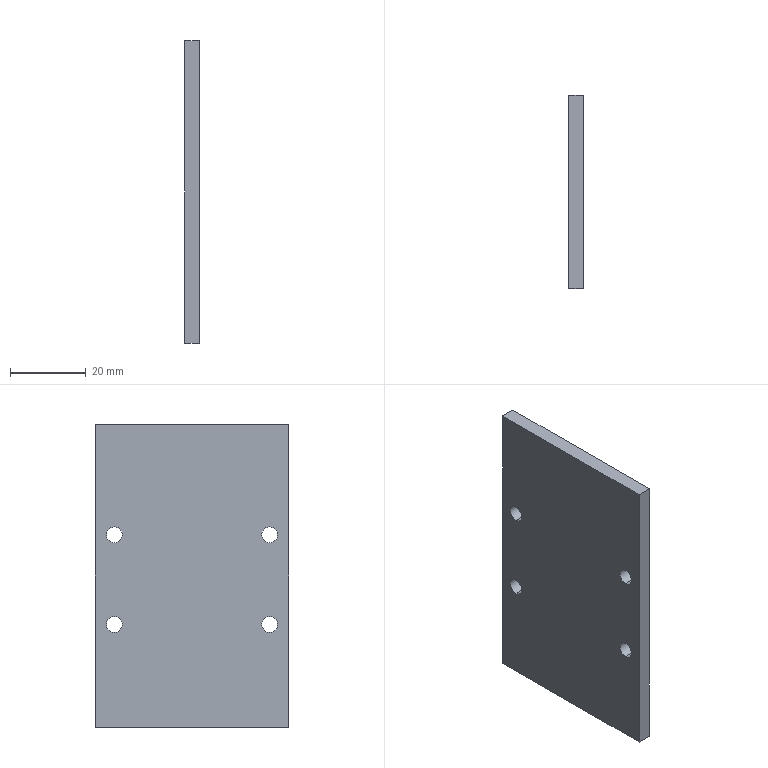Part | SolidWorks | features Cut 1, Extrusion 1 | 1 solid | 14 faces | box 3.85 x 51 x 80 mm | volume 15495 mm3 | cylinder 8 | plane 6 | commonest cylinder face diameters 4.2 x8
STEP:
#1=CARTESIAN_POINT('',(-2.33,-37.544,29.302));
#2=VERTEX_POINT('',#1);
#3=CARTESIAN_POINT('',(-2.33,-37.544,25.102));
#4=VERTEX_POINT('',#3);
#5=CARTESIAN_POINT('',(-2.33,-37.544,27.202));
#6=DIRECTION('',(1.,0.,0.));
#7=DIRECTION('',(0.,1.,0.));
#8=AXIS2_PLACEMENT_3D('',#5,#6,#7);
#9=CIRCLE('',#8,2.1);
#10=EDGE_CURVE('',#2,#4,#9,.T.);
#11=ORIENTED_EDGE('',*,*,#10,.F.);
#12=CARTESIAN_POINT('',(1.52,-37.544,29.302));
#13=VERTEX_POINT('',#12);
#14=CARTESIAN_POINT('',(-18.27,-37.544,29.302));
#15=DIRECTION('',(1.,0.,0.));
#16=VECTOR('',#15,1000.);
#17=LINE('',#14,#16);
#18=EDGE_CURVE('',#2,#13,#17,.T.);
#19=ORIENTED_EDGE('',*,*,#18,.T.);
#20=CARTESIAN_POINT('',(1.52,-37.544,25.102));
#21=VERTEX_POINT('',#20);
#22=CARTESIAN_POINT('',(1.52,-37.544,27.202));
#23=DIRECTION('',(-1.,0.,0.));
#24=DIRECTION('',(0.,-1.,0.));
#25=AXIS2_PLACEMENT_3D('',#22,#23,#24);
#26=CIRCLE('',#25,2.1);
#27=EDGE_CURVE('',#21,#13,#26,.T.);
#28=ORIENTED_EDGE('',*,*,#27,.F.);
#29=CARTESIAN_POINT('',(-18.27,-37.544,25.102));
#30=DIRECTION('',(1.,0.,0.));
#31=VECTOR('',#30,1000.);
#32=LINE('',#29,#31);
#33=EDGE_CURVE('',#4,#21,#32,.T.);
#34=ORIENTED_EDGE('',*,*,#33,.F.);
#35=EDGE_LOOP('',(#11,#19,#28,#34));
#36=FACE_OUTER_BOUND('',#35,.T.);
#37=CARTESIAN_POINT('',(-18.27,-37.544,27.202));
#38=DIRECTION('',(1.,0.,0.));
#39=DIRECTION('',(0.,0.,-1.));
#40=AXIS2_PLACEMENT_3D('',#37,#38,#39);
#41=CYLINDRICAL_SURFACE('',#40,2.1);
#42=ADVANCED_FACE('',(#36),#41,.F.);
#43=CARTESIAN_POINT('',(-2.33,-37.544,52.952));
#44=VERTEX_POINT('',#43);
#45=CARTESIAN_POINT('',(-2.33,-37.544,48.752));
#46=VERTEX_POINT('',#45);
#47=CARTESIAN_POINT('',(-2.33,-37.544,50.852));
#48=DIRECTION('',(1.,0.,0.));
#49=DIRECTION('',(0.,1.,0.));
#50=AXIS2_PLACEMENT_3D('',#47,#48,#49);
#51=CIRCLE('',#50,2.1);
#52=EDGE_CURVE('',#44,#46,#51,.T.);
#53=ORIENTED_EDGE('',*,*,#52,.F.);
#54=CARTESIAN_POINT('',(1.52,-37.544,52.952));
#55=VERTEX_POINT('',#54);
#56=CARTESIAN_POINT('',(-18.27,-37.544,52.952));
#57=DIRECTION('',(1.,0.,0.));
#58=VECTOR('',#57,1000.);
#59=LINE('',#56,#58);
#60=EDGE_CURVE('',#44,#55,#59,.T.);
#61=ORIENTED_EDGE('',*,*,#60,.T.);
#62=CARTESIAN_POINT('',(1.52,-37.544,48.752));
#63=VERTEX_POINT('',#62);
#64=CARTESIAN_POINT('',(1.52,-37.544,50.852));
#65=DIRECTION('',(-1.,0.,0.));
#66=DIRECTION('',(0.,-1.,0.));
#67=AXIS2_PLACEMENT_3D('',#64,#65,#66);
#68=CIRCLE('',#67,2.1);
#69=EDGE_CURVE('',#63,#55,#68,.T.);
#70=ORIENTED_EDGE('',*,*,#69,.F.);
#71=CARTESIAN_POINT('',(-18.27,-37.544,48.752));
#72=DIRECTION('',(1.,0.,0.));
#73=VECTOR('',#72,1000.);
#74=LINE('',#71,#73);
#75=EDGE_CURVE('',#46,#63,#74,.T.);
#76=ORIENTED_EDGE('',*,*,#75,.F.);
#77=EDGE_LOOP('',(#53,#61,#70,#76));
#78=FACE_OUTER_BOUND('',#77,.T.);
#79=CARTESIAN_POINT('',(-18.27,-37.544,50.852));
#80=DIRECTION('',(1.,0.,0.));
#81=DIRECTION('',(0.,0.,-1.));
#82=AXIS2_PLACEMENT_3D('',#79,#80,#81);
#83=CYLINDRICAL_SURFACE('',#82,2.1);
#84=ADVANCED_FACE('',(#78),#83,.F.);
#85=CARTESIAN_POINT('',(-2.33,3.456,52.952));
#86=VERTEX_POINT('',#85);
#87=CARTESIAN_POINT('',(-2.33,3.456,48.752));
#88=VERTEX_POINT('',#87);
#89=CARTESIAN_POINT('',(-2.33,3.456,50.852));
#90=DIRECTION('',(1.,0.,0.));
#91=DIRECTION('',(0.,1.,0.));
#92=AXIS2_PLACEMENT_3D('',#89,#90,#91);
#93=CIRCLE('',#92,2.1);
#94=EDGE_CURVE('',#86,#88,#93,.T.);
#95=ORIENTED_EDGE('',*,*,#94,.F.);
#96=CARTESIAN_POINT('',(1.52,3.456,52.952));
#97=VERTEX_POINT('',#96);
#98=CARTESIAN_POINT('',(-18.27,3.456,52.952));
#99=DIRECTION('',(1.,0.,0.));
#100=VECTOR('',#99,1000.);
#101=LINE('',#98,#100);
#102=EDGE_CURVE('',#86,#97,#101,.T.);
#103=ORIENTED_EDGE('',*,*,#102,.T.);
#104=CARTESIAN_POINT('',(1.52,3.456,48.752));
#105=VERTEX_POINT('',#104);
#106=CARTESIAN_POINT('',(1.52,3.456,50.852));
#107=DIRECTION('',(-1.,0.,0.));
#108=DIRECTION('',(0.,-1.,0.));
#109=AXIS2_PLACEMENT_3D('',#106,#107,#108);
#110=CIRCLE('',#109,2.1);
#111=EDGE_CURVE('',#105,#97,#110,.T.);
#112=ORIENTED_EDGE('',*,*,#111,.F.);
#113=CARTESIAN_POINT('',(-18.27,3.456,48.752));
#114=DIRECTION('',(1.,0.,0.));
#115=VECTOR('',#114,1000.);
#116=LINE('',#113,#115);
#117=EDGE_CURVE('',#88,#105,#116,.T.);
#118=ORIENTED_EDGE('',*,*,#117,.F.);
#119=EDGE_LOOP('',(#95,#103,#112,#118));
#120=FACE_OUTER_BOUND('',#119,.T.);
#121=CARTESIAN_POINT('',(-18.27,3.456,50.852));
#122=DIRECTION('',(1.,0.,0.));
#123=DIRECTION('',(0.,0.,-1.));
#124=AXIS2_PLACEMENT_3D('',#121,#122,#123);
#125=CYLINDRICAL_SURFACE('',#124,2.1);
#126=ADVANCED_FACE('',(#120),#125,.F.);
#127=CARTESIAN_POINT('',(-2.33,3.456,29.302));
#128=VERTEX_POINT('',#127);
#129=CARTESIAN_POINT('',(-2.33,3.456,25.102));
#130=VERTEX_POINT('',#129);
#131=CARTESIAN_POINT('',(-2.33,3.456,27.202));
#132=DIRECTION('',(1.,0.,0.));
#133=DIRECTION('',(0.,1.,0.));
#134=AXIS2_PLACEMENT_3D('',#131,#132,#133);
#135=CIRCLE('',#134,2.1);
#136=EDGE_CURVE('',#128,#130,#135,.T.);
#137=ORIENTED_EDGE('',*,*,#136,.F.);
#138=CARTESIAN_POINT('',(1.52,3.456,29.302));
#139=VERTEX_POINT('',#138);
#140=CARTESIAN_POINT('',(-18.27,3.456,29.302));
#141=DIRECTION('',(1.,0.,0.));
#142=VECTOR('',#141,1000.);
#143=LINE('',#140,#142);
#144=EDGE_CURVE('',#128,#139,#143,.T.);
#145=ORIENTED_EDGE('',*,*,#144,.T.);
#146=CARTESIAN_POINT('',(1.52,3.456,25.102));
#147=VERTEX_POINT('',#146);
#148=CARTESIAN_POINT('',(1.52,3.456,27.202));
#149=DIRECTION('',(-1.,0.,0.));
#150=DIRECTION('',(0.,-1.,0.));
#151=AXIS2_PLACEMENT_3D('',#148,#149,#150);
#152=CIRCLE('',#151,2.1);
#153=EDGE_CURVE('',#147,#139,#152,.T.);
#154=ORIENTED_EDGE('',*,*,#153,.F.);
#155=CARTESIAN_POINT('',(-18.27,3.456,25.102));
#156=DIRECTION('',(1.,0.,0.));
#157=VECTOR('',#156,1000.);
#158=LINE('',#155,#157);
#159=EDGE_CURVE('',#130,#147,#158,.T.);
#160=ORIENTED_EDGE('',*,*,#159,.F.);
#161=EDGE_LOOP('',(#137,#145,#154,#160));
#162=FACE_OUTER_BOUND('',#161,.T.);
#163=CARTESIAN_POINT('',(-18.27,3.456,27.202));
#164=DIRECTION('',(1.,0.,0.));
#165=DIRECTION('',(0.,0.,-1.));
#166=AXIS2_PLACEMENT_3D('',#163,#164,#165);
#167=CYLINDRICAL_SURFACE('',#166,2.1);
#168=ADVANCED_FACE('',(#162),#167,.F.);
#169=CARTESIAN_POINT('',(-2.33,-37.544,27.202));
#170=DIRECTION('',(1.,0.,0.));
#171=DIRECTION('',(0.,1.,0.));
#172=AXIS2_PLACEMENT_3D('',#169,#170,#171);
#173=CIRCLE('',#172,2.1);
#174=EDGE_CURVE('',#4,#2,#173,.T.);
#175=ORIENTED_EDGE('',*,*,#174,.T.);
#176=ORIENTED_EDGE('',*,*,#10,.T.);
#177=EDGE_LOOP('',(#175,#176));
#178=FACE_BOUND('',#177,.T.);
#179=CARTESIAN_POINT('',(-2.33,-37.544,50.852));
#180=DIRECTION('',(1.,0.,0.));
#181=DIRECTION('',(0.,1.,0.));
#182=AXIS2_PLACEMENT_3D('',#179,#180,#181);
#183=CIRCLE('',#182,2.1);
#184=EDGE_CURVE('',#46,#44,#183,.T.);
#185=ORIENTED_EDGE('',*,*,#184,.T.);
#186=ORIENTED_EDGE('',*,*,#52,.T.);
#187=EDGE_LOOP('',(#185,#186));
#188=FACE_BOUND('',#187,.T.);
#189=CARTESIAN_POINT('',(-2.33,3.456,50.852));
#190=DIRECTION('',(1.,0.,0.));
#191=DIRECTION('',(0.,1.,0.));
#192=AXIS2_PLACEMENT_3D('',#189,#190,#191);
#193=CIRCLE('',#192,2.1);
#194=EDGE_CURVE('',#88,#86,#193,.T.);
#195=ORIENTED_EDGE('',*,*,#194,.T.);
#196=ORIENTED_EDGE('',*,*,#94,.T.);
#197=EDGE_LOOP('',(#195,#196));
#198=FACE_BOUND('',#197,.T.);
#199=CARTESIAN_POINT('',(-2.33,3.456,27.202));
#200=DIRECTION('',(1.,0.,0.));
#201=DIRECTION('',(0.,1.,0.));
#202=AXIS2_PLACEMENT_3D('',#199,#200,#201);
#203=CIRCLE('',#202,2.1);
#204=EDGE_CURVE('',#130,#128,#203,.T.);
#205=ORIENTED_EDGE('',*,*,#204,.T.);
#206=ORIENTED_EDGE('',*,*,#136,.T.);
#207=EDGE_LOOP('',(#205,#206));
#208=FACE_BOUND('',#207,.T.);
#209=CARTESIAN_POINT('',(-2.33,8.456,0.));
#210=VERTEX_POINT('',#209);
#211=CARTESIAN_POINT('',(-2.33,-42.544,0.));
#212=VERTEX_POINT('',#211);
#213=CARTESIAN_POINT('',(-2.33,8.456,0.));
#214=DIRECTION('',(0.,-1.,0.));
#215=VECTOR('',#214,1000.);
#216=LINE('',#213,#215);
#217=EDGE_CURVE('',#210,#212,#216,.T.);
#218=ORIENTED_EDGE('',*,*,#217,.T.);
#219=CARTESIAN_POINT('',(-2.33,-42.544,80.));
#220=VERTEX_POINT('',#219);
#221=CARTESIAN_POINT('',(-2.33,-42.544,80.));
#222=DIRECTION('',(0.,0.,-1.));
#223=VECTOR('',#222,1000.);
#224=LINE('',#221,#223);
#225=EDGE_CURVE('',#220,#212,#224,.T.);
#226=ORIENTED_EDGE('',*,*,#225,.F.);
#227=CARTESIAN_POINT('',(-2.33,8.456,80.));
#228=VERTEX_POINT('',#227);
#229=CARTESIAN_POINT('',(-2.33,8.456,80.));
#230=DIRECTION('',(0.,-1.,0.));
#231=VECTOR('',#230,1000.);
#232=LINE('',#229,#231);
#233=EDGE_CURVE('',#228,#220,#232,.T.);
#234=ORIENTED_EDGE('',*,*,#233,.F.);
#235=CARTESIAN_POINT('',(-2.33,8.456,80.));
#236=DIRECTION('',(0.,0.,-1.));
#237=VECTOR('',#236,1000.);
#238=LINE('',#235,#237);
#239=EDGE_CURVE('',#228,#210,#238,.T.);
#240=ORIENTED_EDGE('',*,*,#239,.T.);
#241=EDGE_LOOP('',(#218,#226,#234,#240));
#242=FACE_OUTER_BOUND('',#241,.T.);
#243=CARTESIAN_POINT('',(-2.33,8.456,80.));
#244=DIRECTION('',(1.,0.,0.));
#245=DIRECTION('',(0.,1.,0.));
#246=AXIS2_PLACEMENT_3D('',#243,#244,#245);
#247=PLANE('',#246);
#248=ADVANCED_FACE('',(#178,#188,#198,#208,#242),#247,.F.);
#249=CARTESIAN_POINT('',(1.52,-42.544,0.));
#250=VERTEX_POINT('',#249);
#251=CARTESIAN_POINT('',(-2.33,-42.544,0.));
#252=DIRECTION('',(1.,0.,0.));
#253=VECTOR('',#252,1000.);
#254=LINE('',#251,#253);
#255=EDGE_CURVE('',#212,#250,#254,.T.);
#256=ORIENTED_EDGE('',*,*,#255,.T.);
#257=CARTESIAN_POINT('',(1.52,-42.544,80.));
#258=VERTEX_POINT('',#257);
#259=CARTESIAN_POINT('',(1.52,-42.544,80.));
#260=DIRECTION('',(0.,0.,-1.));
#261=VECTOR('',#260,1000.);
#262=LINE('',#259,#261);
#263=EDGE_CURVE('',#258,#250,#262,.T.);
#264=ORIENTED_EDGE('',*,*,#263,.F.);
#265=CARTESIAN_POINT('',(-2.33,-42.544,80.));
#266=DIRECTION('',(1.,0.,0.));
#267=VECTOR('',#266,1000.);
#268=LINE('',#265,#267);
#269=EDGE_CURVE('',#220,#258,#268,.T.);
#270=ORIENTED_EDGE('',*,*,#269,.F.);
#271=ORIENTED_EDGE('',*,*,#225,.T.);
#272=EDGE_LOOP('',(#256,#264,#270,#271));
#273=FACE_OUTER_BOUND('',#272,.T.);
#274=CARTESIAN_POINT('',(-2.33,-42.544,80.));
#275=DIRECTION('',(0.,1.,0.));
#276=DIRECTION('',(0.,0.,1.));
#277=AXIS2_PLACEMENT_3D('',#274,#275,#276);
#278=PLANE('',#277);
#279=ADVANCED_FACE('',(#273),#278,.F.);
#280=ORIENTED_EDGE('',*,*,#27,.T.);
#281=CARTESIAN_POINT('',(1.52,-37.544,27.202));
#282=DIRECTION('',(-1.,0.,0.));
#283=DIRECTION('',(0.,-1.,0.));
#284=AXIS2_PLACEMENT_3D('',#281,#282,#283);
#285=CIRCLE('',#284,2.1);
#286=EDGE_CURVE('',#13,#21,#285,.T.);
#287=ORIENTED_EDGE('',*,*,#286,.T.);
#288=EDGE_LOOP('',(#280,#287));
#289=FACE_BOUND('',#288,.T.);
#290=ORIENTED_EDGE('',*,*,#69,.T.);
#291=CARTESIAN_POINT('',(1.52,-37.544,50.852));
#292=DIRECTION('',(-1.,0.,0.));
#293=DIRECTION('',(0.,-1.,0.));
#294=AXIS2_PLACEMENT_3D('',#291,#292,#293);
#295=CIRCLE('',#294,2.1);
#296=EDGE_CURVE('',#55,#63,#295,.T.);
#297=ORIENTED_EDGE('',*,*,#296,.T.);
#298=EDGE_LOOP('',(#290,#297));
#299=FACE_BOUND('',#298,.T.);
#300=ORIENTED_EDGE('',*,*,#111,.T.);
#301=CARTESIAN_POINT('',(1.52,3.456,50.852));
#302=DIRECTION('',(-1.,0.,0.));
#303=DIRECTION('',(0.,-1.,0.));
#304=AXIS2_PLACEMENT_3D('',#301,#302,#303);
#305=CIRCLE('',#304,2.1);
#306=EDGE_CURVE('',#97,#105,#305,.T.);
#307=ORIENTED_EDGE('',*,*,#306,.T.);
#308=EDGE_LOOP('',(#300,#307));
#309=FACE_BOUND('',#308,.T.);
#310=ORIENTED_EDGE('',*,*,#153,.T.);
#311=CARTESIAN_POINT('',(1.52,3.456,27.202));
#312=DIRECTION('',(-1.,0.,0.));
#313=DIRECTION('',(0.,-1.,0.));
#314=AXIS2_PLACEMENT_3D('',#311,#312,#313);
#315=CIRCLE('',#314,2.1);
#316=EDGE_CURVE('',#139,#147,#315,.T.);
#317=ORIENTED_EDGE('',*,*,#316,.T.);
#318=EDGE_LOOP('',(#310,#317));
#319=FACE_BOUND('',#318,.T.);
#320=CARTESIAN_POINT('',(1.52,8.456,0.));
#321=VERTEX_POINT('',#320);
#322=CARTESIAN_POINT('',(1.52,8.456,0.));
#323=DIRECTION('',(0.,1.,0.));
#324=VECTOR('',#323,1000.);
#325=LINE('',#322,#324);
#326=EDGE_CURVE('',#250,#321,#325,.T.);
#327=ORIENTED_EDGE('',*,*,#326,.T.);
#328=CARTESIAN_POINT('',(1.52,8.456,80.));
#329=VERTEX_POINT('',#328);
#330=CARTESIAN_POINT('',(1.52,8.456,80.));
#331=DIRECTION('',(0.,0.,-1.));
#332=VECTOR('',#331,1000.);
#333=LINE('',#330,#332);
#334=EDGE_CURVE('',#329,#321,#333,.T.);
#335=ORIENTED_EDGE('',*,*,#334,.F.);
#336=CARTESIAN_POINT('',(1.52,8.456,80.));
#337=DIRECTION('',(0.,1.,0.));
#338=VECTOR('',#337,1000.);
#339=LINE('',#336,#338);
#340=EDGE_CURVE('',#258,#329,#339,.T.);
#341=ORIENTED_EDGE('',*,*,#340,.F.);
#342=ORIENTED_EDGE('',*,*,#263,.T.);
#343=EDGE_LOOP('',(#327,#335,#341,#342));
#344=FACE_OUTER_BOUND('',#343,.T.);
#345=CARTESIAN_POINT('',(1.52,8.456,80.));
#346=DIRECTION('',(-1.,0.,0.));
#347=DIRECTION('',(0.,-1.,0.));
#348=AXIS2_PLACEMENT_3D('',#345,#346,#347);
#349=PLANE('',#348);
#350=ADVANCED_FACE('',(#289,#299,#309,#319,#344),#349,.F.);
#351=CARTESIAN_POINT('',(-2.33,8.456,0.));
#352=DIRECTION('',(-1.,0.,0.));
#353=VECTOR('',#352,1000.);
#354=LINE('',#351,#353);
#355=EDGE_CURVE('',#321,#210,#354,.T.);
#356=ORIENTED_EDGE('',*,*,#355,.T.);
#357=ORIENTED_EDGE('',*,*,#239,.F.);
#358=CARTESIAN_POINT('',(-2.33,8.456,80.));
#359=DIRECTION('',(-1.,0.,0.));
#360=VECTOR('',#359,1000.);
#361=LINE('',#358,#360);
#362=EDGE_CURVE('',#329,#228,#361,.T.);
#363=ORIENTED_EDGE('',*,*,#362,.F.);
#364=ORIENTED_EDGE('',*,*,#334,.T.);
#365=EDGE_LOOP('',(#356,#357,#363,#364));
#366=FACE_OUTER_BOUND('',#365,.T.);
#367=CARTESIAN_POINT('',(-2.33,8.456,80.));
#368=DIRECTION('',(0.,-1.,0.));
#369=DIRECTION('',(0.,0.,-1.));
#370=AXIS2_PLACEMENT_3D('',#367,#368,#369);
#371=PLANE('',#370);
#372=ADVANCED_FACE('',(#366),#371,.F.);
#373=ORIENTED_EDGE('',*,*,#233,.T.);
#374=ORIENTED_EDGE('',*,*,#269,.T.);
#375=ORIENTED_EDGE('',*,*,#340,.T.);
#376=ORIENTED_EDGE('',*,*,#362,.T.);
#377=EDGE_LOOP('',(#373,#374,#375,#376));
#378=FACE_OUTER_BOUND('',#377,.T.);
#379=CARTESIAN_POINT('',(0.,0.,80.));
#380=DIRECTION('',(0.,0.,1.));
#381=DIRECTION('',(1.,0.,0.));
#382=AXIS2_PLACEMENT_3D('',#379,#380,#381);
#383=PLANE('',#382);
#384=ADVANCED_FACE('',(#378),#383,.T.);
#385=ORIENTED_EDGE('',*,*,#217,.F.);
#386=ORIENTED_EDGE('',*,*,#355,.F.);
#387=ORIENTED_EDGE('',*,*,#326,.F.);
#388=ORIENTED_EDGE('',*,*,#255,.F.);
#389=EDGE_LOOP('',(#385,#386,#387,#388));
#390=FACE_OUTER_BOUND('',#389,.T.);
#391=CARTESIAN_POINT('',(0.,0.,0.));
#392=DIRECTION('',(0.,0.,1.));
#393=DIRECTION('',(1.,0.,0.));
#394=AXIS2_PLACEMENT_3D('',#391,#392,#393);
#395=PLANE('',#394);
#396=ADVANCED_FACE('',(#390),#395,.F.);
#397=ORIENTED_EDGE('',*,*,#144,.F.);
#398=ORIENTED_EDGE('',*,*,#204,.F.);
#399=ORIENTED_EDGE('',*,*,#159,.T.);
#400=ORIENTED_EDGE('',*,*,#316,.F.);
#401=EDGE_LOOP('',(#397,#398,#399,#400));
#402=FACE_OUTER_BOUND('',#401,.T.);
#403=CARTESIAN_POINT('',(-18.27,3.456,27.202));
#404=DIRECTION('',(1.,0.,0.));
#405=DIRECTION('',(0.,0.,-1.));
#406=AXIS2_PLACEMENT_3D('',#403,#404,#405);
#407=CYLINDRICAL_SURFACE('',#406,2.1);
#408=ADVANCED_FACE('',(#402),#407,.F.);
#409=ORIENTED_EDGE('',*,*,#102,.F.);
#410=ORIENTED_EDGE('',*,*,#194,.F.);
#411=ORIENTED_EDGE('',*,*,#117,.T.);
#412=ORIENTED_EDGE('',*,*,#306,.F.);
#413=EDGE_LOOP('',(#409,#410,#411,#412));
#414=FACE_OUTER_BOUND('',#413,.T.);
#415=CARTESIAN_POINT('',(-18.27,3.456,50.852));
#416=DIRECTION('',(1.,0.,0.));
#417=DIRECTION('',(0.,0.,-1.));
#418=AXIS2_PLACEMENT_3D('',#415,#416,#417);
#419=CYLINDRICAL_SURFACE('',#418,2.1);
#420=ADVANCED_FACE('',(#414),#419,.F.);
#421=ORIENTED_EDGE('',*,*,#60,.F.);
#422=ORIENTED_EDGE('',*,*,#184,.F.);
#423=ORIENTED_EDGE('',*,*,#75,.T.);
#424=ORIENTED_EDGE('',*,*,#296,.F.);
#425=EDGE_LOOP('',(#421,#422,#423,#424));
#426=FACE_OUTER_BOUND('',#425,.T.);
#427=CARTESIAN_POINT('',(-18.27,-37.544,50.852));
#428=DIRECTION('',(1.,0.,0.));
#429=DIRECTION('',(0.,0.,-1.));
#430=AXIS2_PLACEMENT_3D('',#427,#428,#429);
#431=CYLINDRICAL_SURFACE('',#430,2.1);
#432=ADVANCED_FACE('',(#426),#431,.F.);
#433=ORIENTED_EDGE('',*,*,#18,.F.);
#434=ORIENTED_EDGE('',*,*,#174,.F.);
#435=ORIENTED_EDGE('',*,*,#33,.T.);
#436=ORIENTED_EDGE('',*,*,#286,.F.);
#437=EDGE_LOOP('',(#433,#434,#435,#436));
#438=FACE_OUTER_BOUND('',#437,.T.);
#439=CARTESIAN_POINT('',(-18.27,-37.544,27.202));
#440=DIRECTION('',(1.,0.,0.));
#441=DIRECTION('',(0.,0.,-1.));
#442=AXIS2_PLACEMENT_3D('',#439,#440,#441);
#443=CYLINDRICAL_SURFACE('',#442,2.1);
#444=ADVANCED_FACE('',(#438),#443,.F.);
#445=CLOSED_SHELL('',(#42,#84,#126,#168,#248,#279,#350,#372,#384,#396,#408,#420,#432,#444));
#446=MANIFOLD_SOLID_BREP('',#445);
#447=CARTESIAN_POINT('',(0.,0.,0.));
#448=DIRECTION('',(0.,0.,1.));
#449=DIRECTION('',(1.,0.,0.));
#450=AXIS2_PLACEMENT_3D('',#447,#448,#449);
#451=(LENGTH_UNIT()NAMED_UNIT(*)SI_UNIT(.MILLI.,.METRE.));
#452=UNCERTAINTY_MEASURE_WITH_UNIT(LENGTH_MEASURE(0.00001),#451,'','');
#453=(NAMED_UNIT(*)PLANE_ANGLE_UNIT()SI_UNIT($,.RADIAN.));
#454=(NAMED_UNIT(*)SI_UNIT($,.STERADIAN.)SOLID_ANGLE_UNIT());
#455=(GEOMETRIC_REPRESENTATION_CONTEXT(3)GLOBAL_UNCERTAINTY_ASSIGNED_CONTEXT((#452))GLOBAL_UNIT_ASSIGNED_CONTEXT((#451,#453,#454))REPRESENTATION_CONTEXT('',''));
#456=ADVANCED_BREP_SHAPE_REPRESENTATION('',(#446,#450),#455);